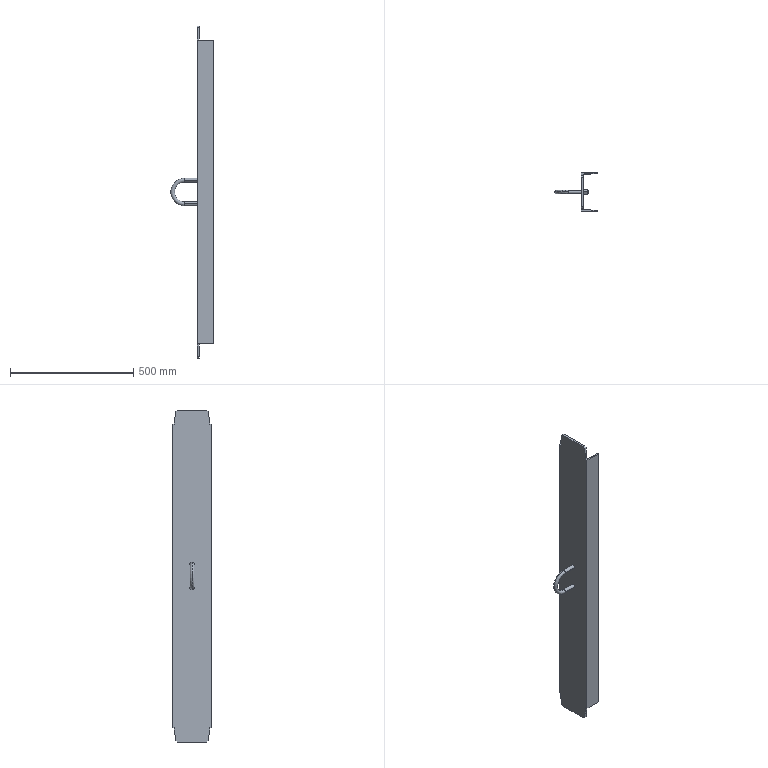Part | SolidWorks | features Chamfer 2, ICE 2, Extrusion 1, HoleWzd 1, MirrorSolid 1, MoveCopyBody 1, Stock 1, Sweep 1 | 4 solids | 66 faces | box 173 x 160 x 1348 mm | volume 2718229 mm3 | plane 40 | cone 12 | cylinder 12 | torus 2 | commonest cylinder face diameters 13.835 x4 16 x4 17 x4